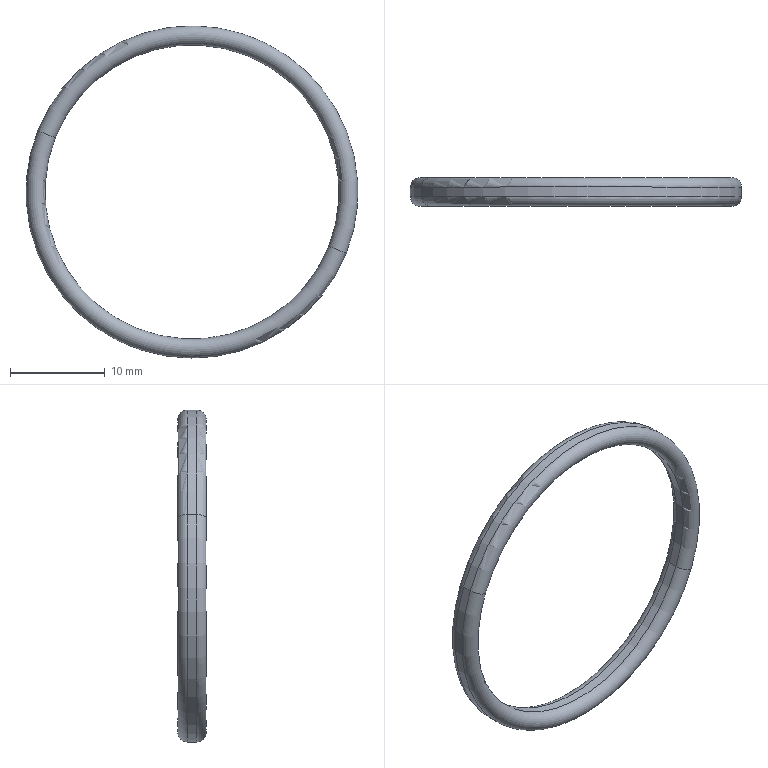Part | SolidWorks | features BaseBody 1 | 1 solid | 8 faces | box 35 x 3 x 35 mm | volume 533.042 mm3 | cylinder 4 | torus 4 | commonest cylinder face diameters 31 x2 35 x2
STEP:
#1=CARTESIAN_POINT('',(245.764,155.1,-6.459));
#2=VERTEX_POINT('',#1);
#3=CARTESIAN_POINT('',(213.236,155.1,6.459));
#4=VERTEX_POINT('',#3);
#5=CARTESIAN_POINT('',(229.5,155.1,0.));
#6=DIRECTION('',(0.,-1.,0.));
#7=DIRECTION('',(0.9294,0.,-0.3691));
#8=AXIS2_PLACEMENT_3D('',#5,#6,#7);
#9=CIRCLE('',#8,17.5);
#10=EDGE_CURVE('',#2,#4,#9,.T.);
#11=ORIENTED_EDGE('',*,*,#10,.T.);
#12=CARTESIAN_POINT('',(213.236,154.1,6.459));
#13=VERTEX_POINT('',#12);
#14=CARTESIAN_POINT('',(213.236,154.6,6.459));
#15=DIRECTION('',(0.,-1.,0.));
#16=VECTOR('',#15,1000.);
#17=LINE('',#14,#16);
#18=EDGE_CURVE('',#4,#13,#17,.T.);
#19=ORIENTED_EDGE('',*,*,#18,.T.);
#20=CARTESIAN_POINT('',(245.764,154.1,-6.459));
#21=VERTEX_POINT('',#20);
#22=CARTESIAN_POINT('',(229.5,154.1,0.));
#23=DIRECTION('',(0.,-1.,0.));
#24=DIRECTION('',(0.9294,0.,-0.3691));
#25=AXIS2_PLACEMENT_3D('',#22,#23,#24);
#26=CIRCLE('',#25,17.5);
#27=EDGE_CURVE('',#21,#13,#26,.T.);
#28=ORIENTED_EDGE('',*,*,#27,.F.);
#29=CARTESIAN_POINT('',(245.764,154.6,-6.459));
#30=DIRECTION('',(0.,-1.,0.));
#31=VECTOR('',#30,1000.);
#32=LINE('',#29,#31);
#33=EDGE_CURVE('',#2,#21,#32,.T.);
#34=ORIENTED_EDGE('',*,*,#33,.F.);
#35=EDGE_LOOP('',(#11,#19,#28,#34));
#36=FACE_OUTER_BOUND('',#35,.T.);
#37=CARTESIAN_POINT('',(229.5,154.6,0.));
#38=DIRECTION('',(0.,-1.,0.));
#39=DIRECTION('',(0.9294,0.,-0.3691));
#40=AXIS2_PLACEMENT_3D('',#37,#38,#39);
#41=CYLINDRICAL_SURFACE('',#40,17.5);
#42=ADVANCED_FACE('',(#36),#41,.T.);
#43=ORIENTED_EDGE('',*,*,#27,.T.);
#44=CARTESIAN_POINT('',(215.095,154.1,5.721));
#45=VERTEX_POINT('',#44);
#46=CARTESIAN_POINT('',(214.165,154.1,6.09));
#47=DIRECTION('',(0.3691,0.,0.9294));
#48=DIRECTION('',(0.9294,0.,-0.3691));
#49=AXIS2_PLACEMENT_3D('',#46,#47,#48);
#50=CIRCLE('',#49,1.);
#51=EDGE_CURVE('',#13,#45,#50,.T.);
#52=ORIENTED_EDGE('',*,*,#51,.T.);
#53=CARTESIAN_POINT('',(243.905,154.1,-5.721));
#54=VERTEX_POINT('',#53);
#55=CARTESIAN_POINT('',(229.5,154.1,0.));
#56=DIRECTION('',(0.,-1.,0.));
#57=DIRECTION('',(0.9294,0.,-0.3691));
#58=AXIS2_PLACEMENT_3D('',#55,#56,#57);
#59=CIRCLE('',#58,15.5);
#60=EDGE_CURVE('',#54,#45,#59,.T.);
#61=ORIENTED_EDGE('',*,*,#60,.F.);
#62=CARTESIAN_POINT('',(244.835,154.1,-6.09));
#63=DIRECTION('',(-0.3691,0.,-0.9294));
#64=DIRECTION('',(-0.9294,0.,0.3691));
#65=AXIS2_PLACEMENT_3D('',#62,#63,#64);
#66=CIRCLE('',#65,1.);
#67=EDGE_CURVE('',#21,#54,#66,.T.);
#68=ORIENTED_EDGE('',*,*,#67,.F.);
#69=EDGE_LOOP('',(#43,#52,#61,#68));
#70=FACE_OUTER_BOUND('',#69,.T.);
#71=CARTESIAN_POINT('',(229.5,154.1,0.));
#72=DIRECTION('',(0.,-1.,0.));
#73=DIRECTION('',(0.9294,0.,-0.3691));
#74=AXIS2_PLACEMENT_3D('',#71,#72,#73);
#75=TOROIDAL_SURFACE('',#74,16.5,1.);
#76=ADVANCED_FACE('',(#70),#75,.T.);
#77=CARTESIAN_POINT('',(215.095,155.1,5.721));
#78=VERTEX_POINT('',#77);
#79=CARTESIAN_POINT('',(243.905,155.1,-5.721));
#80=VERTEX_POINT('',#79);
#81=CARTESIAN_POINT('',(229.5,155.1,0.));
#82=DIRECTION('',(0.,-1.,0.));
#83=DIRECTION('',(0.9294,0.,-0.3691));
#84=AXIS2_PLACEMENT_3D('',#81,#82,#83);
#85=CIRCLE('',#84,15.5);
#86=EDGE_CURVE('',#78,#80,#85,.T.);
#87=ORIENTED_EDGE('',*,*,#86,.F.);
#88=CARTESIAN_POINT('',(215.095,154.6,5.721));
#89=DIRECTION('',(0.,-1.,0.));
#90=VECTOR('',#89,1000.);
#91=LINE('',#88,#90);
#92=EDGE_CURVE('',#78,#45,#91,.T.);
#93=ORIENTED_EDGE('',*,*,#92,.T.);
#94=CARTESIAN_POINT('',(229.5,154.1,0.));
#95=DIRECTION('',(0.,-1.,0.));
#96=DIRECTION('',(0.9294,0.,-0.3691));
#97=AXIS2_PLACEMENT_3D('',#94,#95,#96);
#98=CIRCLE('',#97,15.5);
#99=EDGE_CURVE('',#45,#54,#98,.T.);
#100=ORIENTED_EDGE('',*,*,#99,.T.);
#101=CARTESIAN_POINT('',(243.905,154.6,-5.721));
#102=DIRECTION('',(0.,-1.,0.));
#103=VECTOR('',#102,1000.);
#104=LINE('',#101,#103);
#105=EDGE_CURVE('',#80,#54,#104,.T.);
#106=ORIENTED_EDGE('',*,*,#105,.F.);
#107=EDGE_LOOP('',(#87,#93,#100,#106));
#108=FACE_OUTER_BOUND('',#107,.T.);
#109=CARTESIAN_POINT('',(229.5,154.6,0.));
#110=DIRECTION('',(0.,-1.,0.));
#111=DIRECTION('',(0.9294,0.,-0.3691));
#112=AXIS2_PLACEMENT_3D('',#109,#110,#111);
#113=CYLINDRICAL_SURFACE('',#112,15.5);
#114=ADVANCED_FACE('',(#108),#113,.F.);
#115=CARTESIAN_POINT('',(229.5,155.1,0.));
#116=DIRECTION('',(0.,-1.,0.));
#117=DIRECTION('',(0.9294,0.,-0.3691));
#118=AXIS2_PLACEMENT_3D('',#115,#116,#117);
#119=CIRCLE('',#118,15.5);
#120=EDGE_CURVE('',#80,#78,#119,.T.);
#121=ORIENTED_EDGE('',*,*,#120,.T.);
#122=CARTESIAN_POINT('',(214.165,155.1,6.09));
#123=DIRECTION('',(0.3691,0.,0.9294));
#124=DIRECTION('',(0.9294,0.,-0.3691));
#125=AXIS2_PLACEMENT_3D('',#122,#123,#124);
#126=CIRCLE('',#125,1.);
#127=EDGE_CURVE('',#78,#4,#126,.T.);
#128=ORIENTED_EDGE('',*,*,#127,.T.);
#129=ORIENTED_EDGE('',*,*,#10,.F.);
#130=CARTESIAN_POINT('',(244.835,155.1,-6.09));
#131=DIRECTION('',(-0.3691,0.,-0.9294));
#132=DIRECTION('',(-0.9294,0.,0.3691));
#133=AXIS2_PLACEMENT_3D('',#130,#131,#132);
#134=CIRCLE('',#133,1.);
#135=EDGE_CURVE('',#80,#2,#134,.T.);
#136=ORIENTED_EDGE('',*,*,#135,.F.);
#137=EDGE_LOOP('',(#121,#128,#129,#136));
#138=FACE_OUTER_BOUND('',#137,.T.);
#139=CARTESIAN_POINT('',(229.5,155.1,0.));
#140=DIRECTION('',(0.,-1.,0.));
#141=DIRECTION('',(0.9294,0.,-0.3691));
#142=AXIS2_PLACEMENT_3D('',#139,#140,#141);
#143=TOROIDAL_SURFACE('',#142,16.5,1.);
#144=ADVANCED_FACE('',(#138),#143,.T.);
#145=ORIENTED_EDGE('',*,*,#127,.F.);
#146=ORIENTED_EDGE('',*,*,#86,.T.);
#147=ORIENTED_EDGE('',*,*,#135,.T.);
#148=CARTESIAN_POINT('',(229.5,155.1,0.));
#149=DIRECTION('',(0.,-1.,0.));
#150=DIRECTION('',(0.9294,0.,-0.3691));
#151=AXIS2_PLACEMENT_3D('',#148,#149,#150);
#152=CIRCLE('',#151,17.5);
#153=EDGE_CURVE('',#4,#2,#152,.T.);
#154=ORIENTED_EDGE('',*,*,#153,.F.);
#155=EDGE_LOOP('',(#145,#146,#147,#154));
#156=FACE_OUTER_BOUND('',#155,.T.);
#157=CARTESIAN_POINT('',(229.5,155.1,0.));
#158=DIRECTION('',(0.,-1.,0.));
#159=DIRECTION('',(0.9294,0.,-0.3691));
#160=AXIS2_PLACEMENT_3D('',#157,#158,#159);
#161=TOROIDAL_SURFACE('',#160,16.5,1.);
#162=ADVANCED_FACE('',(#156),#161,.T.);
#163=ORIENTED_EDGE('',*,*,#92,.F.);
#164=ORIENTED_EDGE('',*,*,#120,.F.);
#165=ORIENTED_EDGE('',*,*,#105,.T.);
#166=ORIENTED_EDGE('',*,*,#60,.T.);
#167=EDGE_LOOP('',(#163,#164,#165,#166));
#168=FACE_OUTER_BOUND('',#167,.T.);
#169=CARTESIAN_POINT('',(229.5,154.6,0.));
#170=DIRECTION('',(0.,-1.,0.));
#171=DIRECTION('',(0.9294,0.,-0.3691));
#172=AXIS2_PLACEMENT_3D('',#169,#170,#171);
#173=CYLINDRICAL_SURFACE('',#172,15.5);
#174=ADVANCED_FACE('',(#168),#173,.F.);
#175=ORIENTED_EDGE('',*,*,#51,.F.);
#176=CARTESIAN_POINT('',(229.5,154.1,0.));
#177=DIRECTION('',(0.,-1.,0.));
#178=DIRECTION('',(0.9294,0.,-0.3691));
#179=AXIS2_PLACEMENT_3D('',#176,#177,#178);
#180=CIRCLE('',#179,17.5);
#181=EDGE_CURVE('',#13,#21,#180,.T.);
#182=ORIENTED_EDGE('',*,*,#181,.T.);
#183=ORIENTED_EDGE('',*,*,#67,.T.);
#184=ORIENTED_EDGE('',*,*,#99,.F.);
#185=EDGE_LOOP('',(#175,#182,#183,#184));
#186=FACE_OUTER_BOUND('',#185,.T.);
#187=CARTESIAN_POINT('',(229.5,154.1,0.));
#188=DIRECTION('',(0.,-1.,0.));
#189=DIRECTION('',(0.9294,0.,-0.3691));
#190=AXIS2_PLACEMENT_3D('',#187,#188,#189);
#191=TOROIDAL_SURFACE('',#190,16.5,1.);
#192=ADVANCED_FACE('',(#186),#191,.T.);
#193=ORIENTED_EDGE('',*,*,#18,.F.);
#194=ORIENTED_EDGE('',*,*,#153,.T.);
#195=ORIENTED_EDGE('',*,*,#33,.T.);
#196=ORIENTED_EDGE('',*,*,#181,.F.);
#197=EDGE_LOOP('',(#193,#194,#195,#196));
#198=FACE_OUTER_BOUND('',#197,.T.);
#199=CARTESIAN_POINT('',(229.5,154.6,0.));
#200=DIRECTION('',(0.,-1.,0.));
#201=DIRECTION('',(0.9294,0.,-0.3691));
#202=AXIS2_PLACEMENT_3D('',#199,#200,#201);
#203=CYLINDRICAL_SURFACE('',#202,17.5);
#204=ADVANCED_FACE('',(#198),#203,.T.);
#205=CLOSED_SHELL('',(#42,#76,#114,#144,#162,#174,#192,#204));
#206=MANIFOLD_SOLID_BREP('',#205);
#207=CARTESIAN_POINT('',(0.,0.,0.));
#208=DIRECTION('',(0.,0.,1.));
#209=DIRECTION('',(1.,0.,0.));
#210=AXIS2_PLACEMENT_3D('',#207,#208,#209);
#211=(LENGTH_UNIT()NAMED_UNIT(*)SI_UNIT(.MILLI.,.METRE.));
#212=UNCERTAINTY_MEASURE_WITH_UNIT(LENGTH_MEASURE(0.00001),#211,'','');
#213=(NAMED_UNIT(*)PLANE_ANGLE_UNIT()SI_UNIT($,.RADIAN.));
#214=(NAMED_UNIT(*)SI_UNIT($,.STERADIAN.)SOLID_ANGLE_UNIT());
#215=(GEOMETRIC_REPRESENTATION_CONTEXT(3)GLOBAL_UNCERTAINTY_ASSIGNED_CONTEXT((#212))GLOBAL_UNIT_ASSIGNED_CONTEXT((#211,#213,#214))REPRESENTATION_CONTEXT('',''));
#216=ADVANCED_BREP_SHAPE_REPRESENTATION('',(#206,#210),#215);